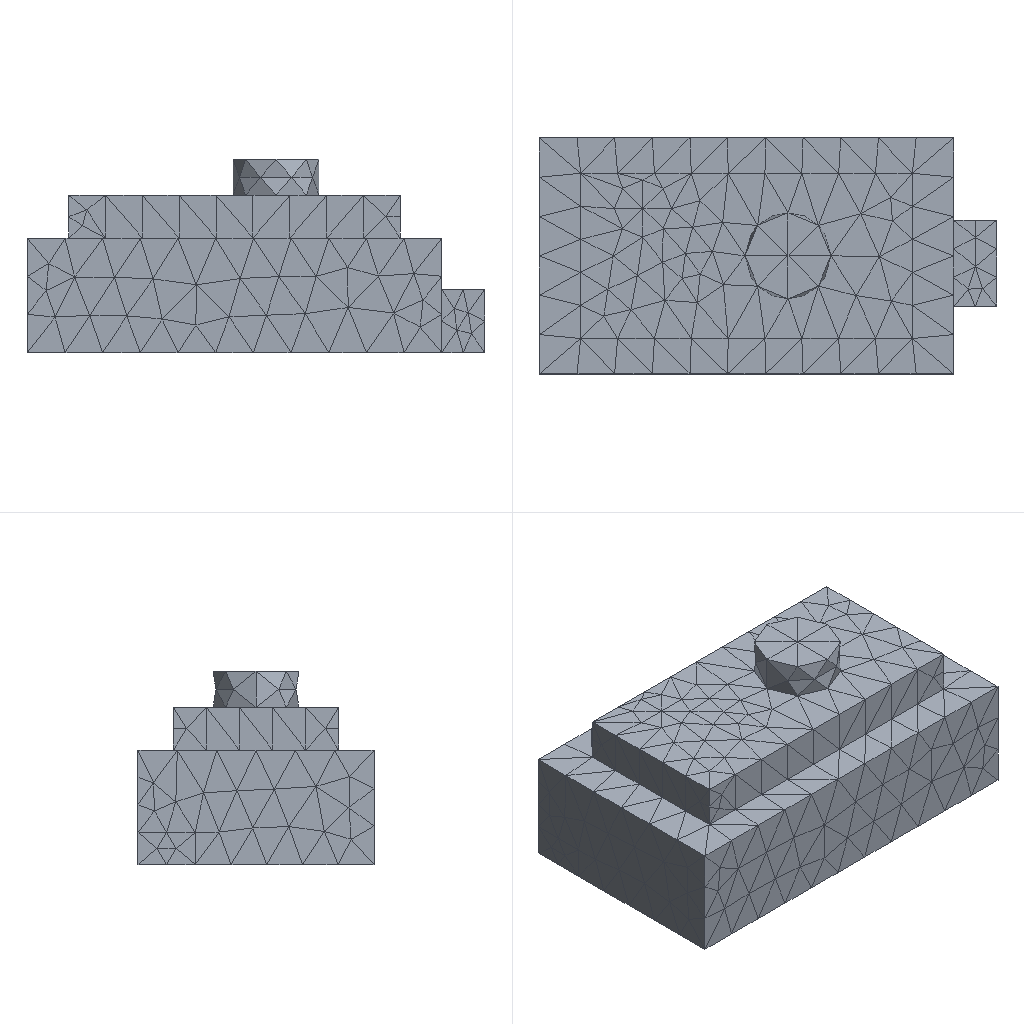Simulation study | ansys mapdl
Set-up summary:
category,name,step,type,value,unit,region
solver,ansys_mapdl
units,mm-N-s-tonne (MPa),,inferred,E=210000 density=
analysis,model,,static
mesh,nodes,,,4239
mesh,elements,,,2528
element_type,SOLID187,,,2528
material,mat 1,,E,210000
material,mat 1,,nu,0.3
load,,model,body load temp,,,all
load,,model,force,"1000 [dir=(0, 0, -1) n=103]",,node list
bc,,model,fixed,"[dofs=UX,UY,UZ n=4699]",,node list
Ansys APDL input file, long lists of numbers shortened:
/COM,ANSYS RELEASE 2026 R1           BUILD 26.1      UP20260202       09:11:09
/PREP7
/NOPR
/TITLE,2
ANTYPE, 0
*IF,_CDRDOFF,EQ,1,THEN     !if solid model was read in
_CDRDOFF=             !reset flag, numoffs already performed
*ELSE              !offset database for the following FE model
NUMOFF,NODE,     4239
NUMOFF,ELEM,     2528
NUMOFF,MAT ,        1
NUMOFF,TYPE,        1
*ENDIF
*SET,_RETURN ,  0.
*SET,_STATUS ,  0.
*SET,_UIQR   ,  103.
*SET,__FLOATPARAMETER__,  4239.
DOF,DELETE
ETBLOCK,        1,        1
(2i9,19a9)
        1      187        0        0        0        0        0        0        0        0        0        0        0        0        0        0        0        0        0        0        0
       -1
NBLOCK,6,SOLID,      4239,      4239
(3i9,6e21.13e3)
        1        0        0-4.1950000000000E+001 3.3000000000000E+001 9.0000000000000E+000
! (4238 more lines like these left out)
N,UNBL,LOC,       -1,
EBLOCK,19,SOLID,      2528,      2528
(19i10)
         1         1         1         1         0         0         0         0        10         0         1      1651      1652      1653      1654      1887      1888      1889      1890
! (5055 more lines like these left out)
        -1
MPTEMP,UNBL, 1, 1,  0.    ,
MPDATA,UNBL, 1,EX  ,       1, 1,  210000.000    ,
MPTEMP,UNBL, 1, 1,  0.    ,
MPDATA,UNBL, 1,NUXY,       1, 1, 0.3    ,
MPTEMP,UNBL, 1, 1,  0.    ,
MPDATA,UNBL, 1,PRXY,       1, 1, 0.3    ,
EXTOPT,ATTR,      0,      0,      0
EXTOPT,ESIZE,  0,  0.
EXTOPT,ACLEAR,      0
TREF,  0.
IRLF,  0
BFUNIF,TEMP,_TINY
ACEL,  0.    ,  0.    ,  0.
OMEGA,  0.    ,  0.    ,  0.
DOMEGA,  0.    ,  0.    ,  0.
CGLOC,  0.    ,  0.    ,  0.
CGOMEGA,  0.    ,  0.    ,  0.
DCGOMG,  0.    ,  0.    ,  0.
KUSE,     0
TIME,  0.
ALPHAD,  0.
BETAD,  0.
DMPRAT,  0.
DMPSTR,  0.
CRPLIM, 0.1    ,   0
CRPLIM,  0.    ,   1
NCNV,     0, 1.000000000E+12,     0,  0.    ,  0.
NEQIT,     0
ERESX,DEFA
DBLOCK,      4699
(i9,a6,2(pg16.9))
        1  UX    0.00000000      0.00000000
! (4698 more lines like these left out)
       -1
FBLOCK,       103
(i9,a6,2(pg16.9))
      794  FZ   -9.70873786      0.00000000
! (102 more lines like these left out)
       -1
/GO
FINISH
Results summary:
result,analysis_type_db,,,static,unstated
result,n_sets,,,1,unstated
result,load_steps[0].set,load_step=1,,1,unstated
result,load_steps[0].substep,load_step=1,,1,unstated
result,load_steps[0].time,load_step=1,,1,unstated
result,load_steps[0].freq,load_step=1,,1,unstated
result,load_steps[0].max_usum,load_step=1,,0.0002649,unstated
result,load_steps[0].max_seqv,load_step=1,,3.108,unstated
result,load_steps[0].reaction_sum.FX,load_step=1,,2.83472e-12,unstated
result,load_steps[0].reaction_sum.FY,load_step=1,,-1.01226e-11,unstated
result,load_steps[0].reaction_sum.FZ,load_step=1,,1000,unstated
result,load_steps[0].reaction_sum.MX,load_step=1,,0,unstated
result,load_steps[0].reaction_sum.MY,load_step=1,,0,unstated
result,load_steps[0].reaction_sum.MZ,load_step=1,,0,unstated
result,convergence,,,results present for all listed sets,unstated